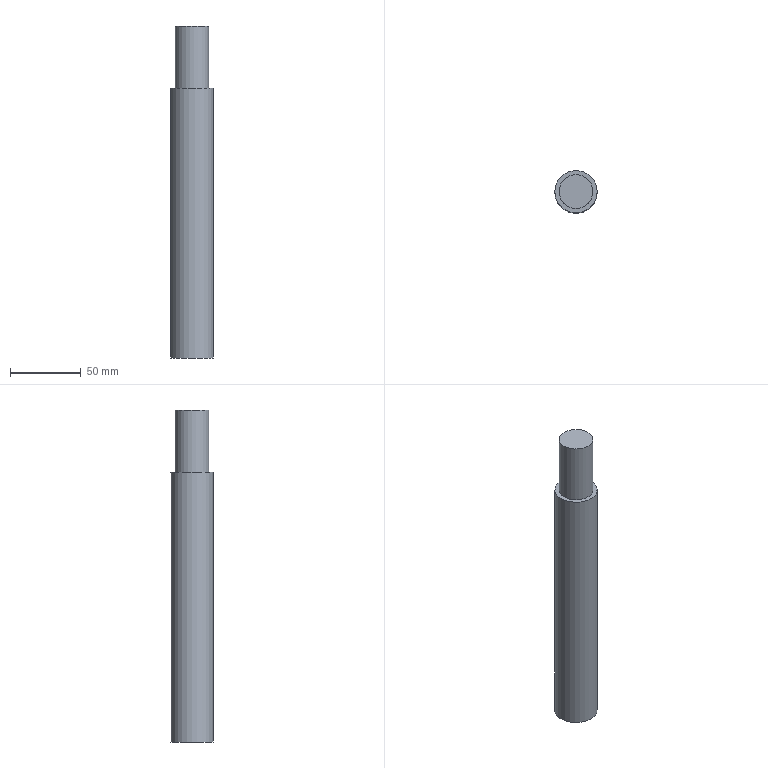Part | NX | features solid 2 | 1 solid | 5 faces | box 30 x 30 x 235 mm | volume 154915 mm3 | plane 3 | cylinder 2 | commonest cylinder face diameters 24 x1 30 x1
STEP:
#1=CARTESIAN_POINT('',(40.,77.5,-59.));
#2=VERTEX_POINT('',#1);
#3=CARTESIAN_POINT('',(55.,77.5,-59.));
#4=DIRECTION('',(0.,0.,-1.));
#5=DIRECTION('',(-1.,0.,0.));
#6=AXIS2_PLACEMENT_3D('',#3,#4,#5);
#7=CIRCLE('',#6,15.);
#8=EDGE_CURVE('',#2,#2,#7,.T.);
#9=ORIENTED_EDGE('',*,*,#8,.F.);
#10=EDGE_LOOP('',(#9));
#11=FACE_BOUND('',#10,.T.);
#12=CARTESIAN_POINT('',(43.,77.5,-59.));
#13=VERTEX_POINT('',#12);
#14=CARTESIAN_POINT('',(55.,77.5,-59.));
#15=DIRECTION('',(0.,0.,-1.));
#16=DIRECTION('',(-1.,0.,0.));
#17=AXIS2_PLACEMENT_3D('',#14,#15,#16);
#18=CIRCLE('',#17,12.);
#19=EDGE_CURVE('',#13,#13,#18,.T.);
#20=ORIENTED_EDGE('',*,*,#19,.T.);
#21=EDGE_LOOP('',(#20));
#22=FACE_BOUND('',#21,.T.);
#23=CARTESIAN_POINT('',(55.,77.5,-59.));
#24=DIRECTION('',(0.,0.,1.));
#25=DIRECTION('',(-1.,0.,0.));
#26=AXIS2_PLACEMENT_3D('',#23,#24,#25);
#27=PLANE('',#26);
#28=ADVANCED_FACE('',(#11,#22),#27,.T.);
#29=CARTESIAN_POINT('',(40.,77.5,-250.));
#30=VERTEX_POINT('',#29);
#31=CARTESIAN_POINT('',(55.,77.5,-250.));
#32=DIRECTION('',(0.,0.,-1.));
#33=DIRECTION('',(-1.,0.,0.));
#34=AXIS2_PLACEMENT_3D('',#31,#32,#33);
#35=CIRCLE('',#34,15.);
#36=EDGE_CURVE('',#30,#30,#35,.T.);
#37=ORIENTED_EDGE('',*,*,#36,.F.);
#38=EDGE_LOOP('',(#37));
#39=FACE_BOUND('',#38,.T.);
#40=ORIENTED_EDGE('',*,*,#8,.T.);
#41=EDGE_LOOP('',(#40));
#42=FACE_BOUND('',#41,.T.);
#43=CARTESIAN_POINT('',(55.,77.5,-250.));
#44=DIRECTION('',(0.,0.,1.));
#45=DIRECTION('',(-1.,0.,0.));
#46=AXIS2_PLACEMENT_3D('',#43,#44,#45);
#47=CYLINDRICAL_SURFACE('',#46,15.);
#48=ADVANCED_FACE('',(#39,#42),#47,.T.);
#49=ORIENTED_EDGE('',*,*,#36,.T.);
#50=EDGE_LOOP('',(#49));
#51=FACE_BOUND('',#50,.T.);
#52=CARTESIAN_POINT('',(55.,77.5,-250.));
#53=DIRECTION('',(0.,0.,1.));
#54=DIRECTION('',(-1.,0.,0.));
#55=AXIS2_PLACEMENT_3D('',#52,#53,#54);
#56=PLANE('',#55);
#57=ADVANCED_FACE('',(#51),#56,.F.);
#58=CARTESIAN_POINT('',(43.,77.5,-15.));
#59=VERTEX_POINT('',#58);
#60=CARTESIAN_POINT('',(55.,77.5,-15.));
#61=DIRECTION('',(0.,0.,-1.));
#62=DIRECTION('',(-1.,0.,0.));
#63=AXIS2_PLACEMENT_3D('',#60,#61,#62);
#64=CIRCLE('',#63,12.);
#65=EDGE_CURVE('',#59,#59,#64,.T.);
#66=ORIENTED_EDGE('',*,*,#65,.T.);
#67=EDGE_LOOP('',(#66));
#68=FACE_BOUND('',#67,.T.);
#69=ORIENTED_EDGE('',*,*,#19,.F.);
#70=EDGE_LOOP('',(#69));
#71=FACE_BOUND('',#70,.T.);
#72=CARTESIAN_POINT('',(55.,77.5,-10.));
#73=DIRECTION('',(0.,0.,-1.));
#74=DIRECTION('',(1.,0.,0.));
#75=AXIS2_PLACEMENT_3D('',#72,#73,#74);
#76=CYLINDRICAL_SURFACE('',#75,12.);
#77=ADVANCED_FACE('',(#68,#71),#76,.T.);
#78=ORIENTED_EDGE('',*,*,#65,.F.);
#79=EDGE_LOOP('',(#78));
#80=FACE_BOUND('',#79,.T.);
#81=CARTESIAN_POINT('',(55.,77.5,-15.));
#82=DIRECTION('',(0.,0.,1.));
#83=DIRECTION('',(-1.,0.,0.));
#84=AXIS2_PLACEMENT_3D('',#81,#82,#83);
#85=PLANE('',#84);
#86=ADVANCED_FACE('',(#80),#85,.T.);
#87=CLOSED_SHELL('',(#28,#48,#57,#77,#86));
#88=MANIFOLD_SOLID_BREP('',#87);
#89=(LENGTH_UNIT()NAMED_UNIT(*)SI_UNIT(.MILLI.,.METRE.));
#90=UNCERTAINTY_MEASURE_WITH_UNIT(LENGTH_MEASURE(0.00001),#89,'','');
#91=(NAMED_UNIT(*)PLANE_ANGLE_UNIT()SI_UNIT($,.RADIAN.));
#92=(NAMED_UNIT(*)SI_UNIT($,.STERADIAN.)SOLID_ANGLE_UNIT());
#93=(GEOMETRIC_REPRESENTATION_CONTEXT(3)GLOBAL_UNCERTAINTY_ASSIGNED_CONTEXT((#90))GLOBAL_UNIT_ASSIGNED_CONTEXT((#89,#91,#92))REPRESENTATION_CONTEXT('',''));
#94=ADVANCED_BREP_SHAPE_REPRESENTATION('',(#88),#93);